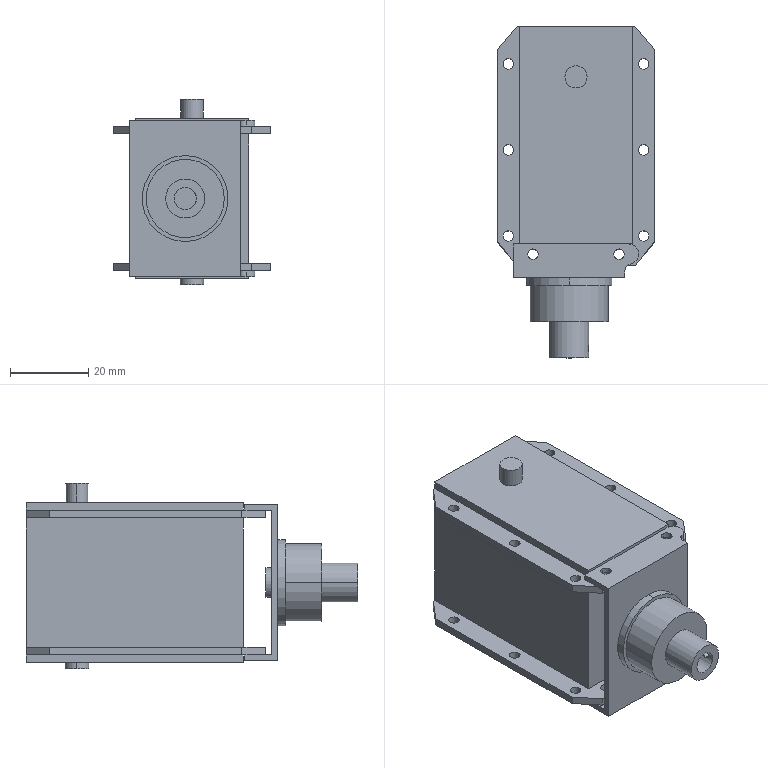Part | SolidWorks | 4 solids | 167 faces | box 40.2 x 84.8 x 47.35 mm | volume 75606 mm3 | cylinder 108 | plane 59 | commonest cylinder face diameters 2.7 x40 2 x34 6 x6 3 x4 5.7 x4 3.2 x2